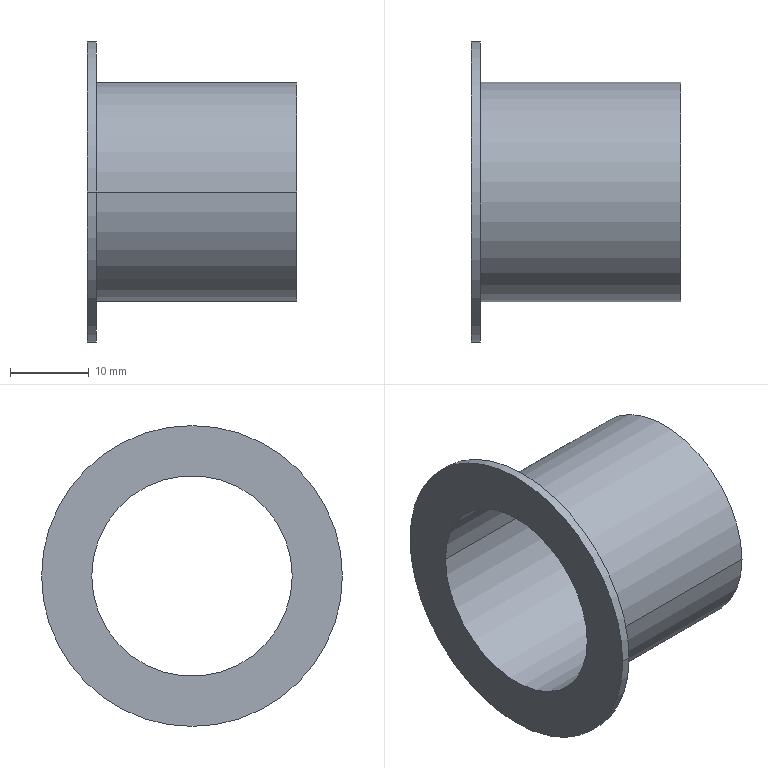Part | NX | features BREP 1 | 1 solid | 9 faces | box 26.543 x 38.1 x 38.1 mm | volume 3243 mm3 | cylinder 6 | plane 3 | commonest cylinder face diameters 25.4 x2 27.775 x2 38.1 x2
STEP:
#1=CARTESIAN_POINT('',(0.,19.05,0.));
#2=VERTEX_POINT('',#1);
#3=CARTESIAN_POINT('',(0.,-19.05,0.));
#4=VERTEX_POINT('',#3);
#5=CARTESIAN_POINT('',(0.,0.,0.));
#6=DIRECTION('',(1.,0.,0.));
#7=DIRECTION('',(0.,1.,0.));
#8=AXIS2_PLACEMENT_3D('',#5,#6,#7);
#9=CIRCLE('',#8,19.05);
#10=EDGE_CURVE('',#2,#4,#9,.T.);
#11=ORIENTED_EDGE('',*,*,#10,.F.);
#12=CARTESIAN_POINT('',(0.,0.,0.));
#13=DIRECTION('',(-1.,0.,0.));
#14=DIRECTION('',(0.,1.,0.));
#15=AXIS2_PLACEMENT_3D('',#12,#13,#14);
#16=CIRCLE('',#15,19.05);
#17=EDGE_CURVE('',#2,#4,#16,.T.);
#18=ORIENTED_EDGE('',*,*,#17,.T.);
#19=EDGE_LOOP('',(#11,#18));
#20=FACE_BOUND('',#19,.T.);
#21=CARTESIAN_POINT('',(0.,12.7,0.));
#22=VERTEX_POINT('',#21);
#23=CARTESIAN_POINT('',(0.,-12.7,0.));
#24=VERTEX_POINT('',#23);
#25=CARTESIAN_POINT('',(0.,0.,0.));
#26=DIRECTION('',(-1.,0.,0.));
#27=DIRECTION('',(0.,1.,0.));
#28=AXIS2_PLACEMENT_3D('',#25,#26,#27);
#29=CIRCLE('',#28,12.7);
#30=EDGE_CURVE('',#22,#24,#29,.T.);
#31=ORIENTED_EDGE('',*,*,#30,.F.);
#32=CARTESIAN_POINT('',(0.,0.,0.));
#33=DIRECTION('',(1.,0.,0.));
#34=DIRECTION('',(0.,1.,0.));
#35=AXIS2_PLACEMENT_3D('',#32,#33,#34);
#36=CIRCLE('',#35,12.7);
#37=EDGE_CURVE('',#22,#24,#36,.T.);
#38=ORIENTED_EDGE('',*,*,#37,.T.);
#39=EDGE_LOOP('',(#31,#38));
#40=FACE_BOUND('',#39,.T.);
#41=CARTESIAN_POINT('',(0.,0.,0.));
#42=DIRECTION('',(1.,0.,0.));
#43=DIRECTION('',(0.,1.,0.));
#44=AXIS2_PLACEMENT_3D('',#41,#42,#43);
#45=PLANE('',#44);
#46=ADVANCED_FACE('',(#20,#40),#45,.F.);
#47=CARTESIAN_POINT('',(26.543,12.7,0.));
#48=VERTEX_POINT('',#47);
#49=CARTESIAN_POINT('',(26.543,-12.7,0.));
#50=VERTEX_POINT('',#49);
#51=CARTESIAN_POINT('',(26.543,0.,0.));
#52=DIRECTION('',(1.,0.,0.));
#53=DIRECTION('',(0.,1.,0.));
#54=AXIS2_PLACEMENT_3D('',#51,#52,#53);
#55=CIRCLE('',#54,12.7);
#56=EDGE_CURVE('',#48,#50,#55,.T.);
#57=ORIENTED_EDGE('',*,*,#56,.T.);
#58=CARTESIAN_POINT('',(0.,-12.7,0.));
#59=DIRECTION('',(1.,0.,0.));
#60=VECTOR('',#59,1000.);
#61=LINE('',#58,#60);
#62=EDGE_CURVE('',#50,#24,#61,.F.);
#63=ORIENTED_EDGE('',*,*,#62,.T.);
#64=ORIENTED_EDGE('',*,*,#37,.F.);
#65=CARTESIAN_POINT('',(0.,12.7,0.));
#66=DIRECTION('',(1.,0.,0.));
#67=VECTOR('',#66,1000.);
#68=LINE('',#65,#67);
#69=EDGE_CURVE('',#48,#22,#68,.F.);
#70=ORIENTED_EDGE('',*,*,#69,.F.);
#71=EDGE_LOOP('',(#57,#63,#64,#70));
#72=FACE_BOUND('',#71,.T.);
#73=CARTESIAN_POINT('',(-1.327,0.,0.));
#74=DIRECTION('',(1.,0.,0.));
#75=DIRECTION('',(0.,-1.,0.));
#76=AXIS2_PLACEMENT_3D('',#73,#74,#75);
#77=CYLINDRICAL_SURFACE('',#76,12.7);
#78=ADVANCED_FACE('',(#72),#77,.F.);
#79=ORIENTED_EDGE('',*,*,#30,.T.);
#80=ORIENTED_EDGE('',*,*,#62,.F.);
#81=CARTESIAN_POINT('',(26.543,0.,0.));
#82=DIRECTION('',(-1.,0.,0.));
#83=DIRECTION('',(0.,1.,0.));
#84=AXIS2_PLACEMENT_3D('',#81,#82,#83);
#85=CIRCLE('',#84,12.7);
#86=EDGE_CURVE('',#48,#50,#85,.T.);
#87=ORIENTED_EDGE('',*,*,#86,.F.);
#88=ORIENTED_EDGE('',*,*,#69,.T.);
#89=EDGE_LOOP('',(#79,#80,#87,#88));
#90=FACE_BOUND('',#89,.T.);
#91=CARTESIAN_POINT('',(-1.327,0.,0.));
#92=DIRECTION('',(1.,0.,0.));
#93=DIRECTION('',(0.,-1.,0.));
#94=AXIS2_PLACEMENT_3D('',#91,#92,#93);
#95=CYLINDRICAL_SURFACE('',#94,12.7);
#96=ADVANCED_FACE('',(#90),#95,.F.);
#97=CARTESIAN_POINT('',(26.543,13.887,0.));
#98=VERTEX_POINT('',#97);
#99=CARTESIAN_POINT('',(26.543,-13.887,0.));
#100=VERTEX_POINT('',#99);
#101=CARTESIAN_POINT('',(26.543,0.,0.));
#102=DIRECTION('',(-1.,0.,0.));
#103=DIRECTION('',(0.,1.,0.));
#104=AXIS2_PLACEMENT_3D('',#101,#102,#103);
#105=CIRCLE('',#104,13.887);
#106=EDGE_CURVE('',#98,#100,#105,.T.);
#107=ORIENTED_EDGE('',*,*,#106,.F.);
#108=CARTESIAN_POINT('',(26.543,0.,0.));
#109=DIRECTION('',(1.,0.,0.));
#110=DIRECTION('',(0.,1.,0.));
#111=AXIS2_PLACEMENT_3D('',#108,#109,#110);
#112=CIRCLE('',#111,13.887);
#113=EDGE_CURVE('',#98,#100,#112,.T.);
#114=ORIENTED_EDGE('',*,*,#113,.T.);
#115=EDGE_LOOP('',(#107,#114));
#116=FACE_BOUND('',#115,.T.);
#117=ORIENTED_EDGE('',*,*,#56,.F.);
#118=ORIENTED_EDGE('',*,*,#86,.T.);
#119=EDGE_LOOP('',(#117,#118));
#120=FACE_BOUND('',#119,.T.);
#121=CARTESIAN_POINT('',(26.543,0.,0.));
#122=DIRECTION('',(1.,0.,0.));
#123=DIRECTION('',(0.,1.,0.));
#124=AXIS2_PLACEMENT_3D('',#121,#122,#123);
#125=PLANE('',#124);
#126=ADVANCED_FACE('',(#116,#120),#125,.T.);
#127=CARTESIAN_POINT('',(1.143,13.887,0.));
#128=VERTEX_POINT('',#127);
#129=CARTESIAN_POINT('',(1.143,-13.887,0.));
#130=VERTEX_POINT('',#129);
#131=CARTESIAN_POINT('',(1.143,0.,0.));
#132=DIRECTION('',(1.,0.,0.));
#133=DIRECTION('',(0.,1.,0.));
#134=AXIS2_PLACEMENT_3D('',#131,#132,#133);
#135=CIRCLE('',#134,13.887);
#136=EDGE_CURVE('',#128,#130,#135,.T.);
#137=ORIENTED_EDGE('',*,*,#136,.T.);
#138=CARTESIAN_POINT('',(26.543,-13.887,0.));
#139=DIRECTION('',(-1.,0.,0.));
#140=VECTOR('',#139,1000.);
#141=LINE('',#138,#140);
#142=EDGE_CURVE('',#130,#100,#141,.F.);
#143=ORIENTED_EDGE('',*,*,#142,.T.);
#144=ORIENTED_EDGE('',*,*,#113,.F.);
#145=CARTESIAN_POINT('',(26.543,13.887,0.));
#146=DIRECTION('',(-1.,0.,0.));
#147=VECTOR('',#146,1000.);
#148=LINE('',#145,#147);
#149=EDGE_CURVE('',#128,#98,#148,.F.);
#150=ORIENTED_EDGE('',*,*,#149,.F.);
#151=EDGE_LOOP('',(#137,#143,#144,#150));
#152=FACE_BOUND('',#151,.T.);
#153=CARTESIAN_POINT('',(-1.327,0.,0.));
#154=DIRECTION('',(1.,0.,0.));
#155=DIRECTION('',(0.,-1.,0.));
#156=AXIS2_PLACEMENT_3D('',#153,#154,#155);
#157=CYLINDRICAL_SURFACE('',#156,13.887);
#158=ADVANCED_FACE('',(#152),#157,.T.);
#159=ORIENTED_EDGE('',*,*,#106,.T.);
#160=ORIENTED_EDGE('',*,*,#142,.F.);
#161=CARTESIAN_POINT('',(1.143,0.,0.));
#162=DIRECTION('',(-1.,0.,0.));
#163=DIRECTION('',(0.,1.,0.));
#164=AXIS2_PLACEMENT_3D('',#161,#162,#163);
#165=CIRCLE('',#164,13.887);
#166=EDGE_CURVE('',#128,#130,#165,.T.);
#167=ORIENTED_EDGE('',*,*,#166,.F.);
#168=ORIENTED_EDGE('',*,*,#149,.T.);
#169=EDGE_LOOP('',(#159,#160,#167,#168));
#170=FACE_BOUND('',#169,.T.);
#171=CARTESIAN_POINT('',(-1.327,0.,0.));
#172=DIRECTION('',(1.,0.,0.));
#173=DIRECTION('',(0.,-1.,0.));
#174=AXIS2_PLACEMENT_3D('',#171,#172,#173);
#175=CYLINDRICAL_SURFACE('',#174,13.887);
#176=ADVANCED_FACE('',(#170),#175,.T.);
#177=CARTESIAN_POINT('',(1.143,19.05,0.));
#178=VERTEX_POINT('',#177);
#179=CARTESIAN_POINT('',(1.143,-19.05,0.));
#180=VERTEX_POINT('',#179);
#181=CARTESIAN_POINT('',(1.143,0.,0.));
#182=DIRECTION('',(-1.,0.,0.));
#183=DIRECTION('',(0.,1.,0.));
#184=AXIS2_PLACEMENT_3D('',#181,#182,#183);
#185=CIRCLE('',#184,19.05);
#186=EDGE_CURVE('',#178,#180,#185,.T.);
#187=ORIENTED_EDGE('',*,*,#186,.F.);
#188=CARTESIAN_POINT('',(1.143,0.,0.));
#189=DIRECTION('',(1.,0.,0.));
#190=DIRECTION('',(0.,1.,0.));
#191=AXIS2_PLACEMENT_3D('',#188,#189,#190);
#192=CIRCLE('',#191,19.05);
#193=EDGE_CURVE('',#178,#180,#192,.T.);
#194=ORIENTED_EDGE('',*,*,#193,.T.);
#195=EDGE_LOOP('',(#187,#194));
#196=FACE_BOUND('',#195,.T.);
#197=ORIENTED_EDGE('',*,*,#136,.F.);
#198=ORIENTED_EDGE('',*,*,#166,.T.);
#199=EDGE_LOOP('',(#197,#198));
#200=FACE_BOUND('',#199,.T.);
#201=CARTESIAN_POINT('',(1.143,0.,0.));
#202=DIRECTION('',(1.,0.,0.));
#203=DIRECTION('',(0.,1.,0.));
#204=AXIS2_PLACEMENT_3D('',#201,#202,#203);
#205=PLANE('',#204);
#206=ADVANCED_FACE('',(#196,#200),#205,.T.);
#207=ORIENTED_EDGE('',*,*,#10,.T.);
#208=CARTESIAN_POINT('',(1.143,-19.05,0.));
#209=DIRECTION('',(-1.,0.,0.));
#210=VECTOR('',#209,1000.);
#211=LINE('',#208,#210);
#212=EDGE_CURVE('',#4,#180,#211,.F.);
#213=ORIENTED_EDGE('',*,*,#212,.T.);
#214=ORIENTED_EDGE('',*,*,#193,.F.);
#215=CARTESIAN_POINT('',(1.143,19.05,0.));
#216=DIRECTION('',(-1.,0.,0.));
#217=VECTOR('',#216,1000.);
#218=LINE('',#215,#217);
#219=EDGE_CURVE('',#2,#178,#218,.F.);
#220=ORIENTED_EDGE('',*,*,#219,.F.);
#221=EDGE_LOOP('',(#207,#213,#214,#220));
#222=FACE_BOUND('',#221,.T.);
#223=CARTESIAN_POINT('',(-1.327,0.,0.));
#224=DIRECTION('',(1.,0.,0.));
#225=DIRECTION('',(0.,-1.,0.));
#226=AXIS2_PLACEMENT_3D('',#223,#224,#225);
#227=CYLINDRICAL_SURFACE('',#226,19.05);
#228=ADVANCED_FACE('',(#222),#227,.T.);
#229=ORIENTED_EDGE('',*,*,#186,.T.);
#230=ORIENTED_EDGE('',*,*,#212,.F.);
#231=ORIENTED_EDGE('',*,*,#17,.F.);
#232=ORIENTED_EDGE('',*,*,#219,.T.);
#233=EDGE_LOOP('',(#229,#230,#231,#232));
#234=FACE_BOUND('',#233,.T.);
#235=CARTESIAN_POINT('',(-1.327,0.,0.));
#236=DIRECTION('',(1.,0.,0.));
#237=DIRECTION('',(0.,-1.,0.));
#238=AXIS2_PLACEMENT_3D('',#235,#236,#237);
#239=CYLINDRICAL_SURFACE('',#238,19.05);
#240=ADVANCED_FACE('',(#234),#239,.T.);
#241=CLOSED_SHELL('',(#46,#78,#96,#126,#158,#176,#206,#228,#240));
#242=MANIFOLD_SOLID_BREP('',#241);
#243=(LENGTH_UNIT()NAMED_UNIT(*)SI_UNIT(.MILLI.,.METRE.));
#244=UNCERTAINTY_MEASURE_WITH_UNIT(LENGTH_MEASURE(0.00001),#243,'','');
#245=(NAMED_UNIT(*)PLANE_ANGLE_UNIT()SI_UNIT($,.RADIAN.));
#246=(NAMED_UNIT(*)SI_UNIT($,.STERADIAN.)SOLID_ANGLE_UNIT());
#247=(GEOMETRIC_REPRESENTATION_CONTEXT(3)GLOBAL_UNCERTAINTY_ASSIGNED_CONTEXT((#244))GLOBAL_UNIT_ASSIGNED_CONTEXT((#243,#245,#246))REPRESENTATION_CONTEXT('',''));
#248=ADVANCED_BREP_SHAPE_REPRESENTATION('',(#242),#247);